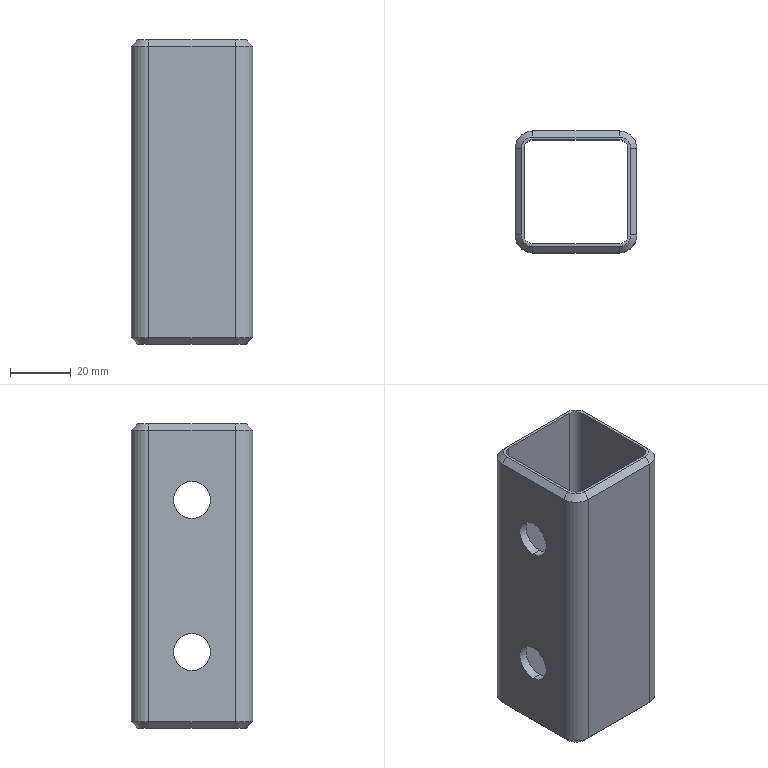Part | STEP file | IN-01-01-04-04 | 1 solid | 42 faces | box 40 x 40 x 100 mm | volume 38931 mm3 | plane 18 | cylinder 16 | cone 8 | commonest cylinder face diameters 12.2 x8 5.8 x4 11.6 x4